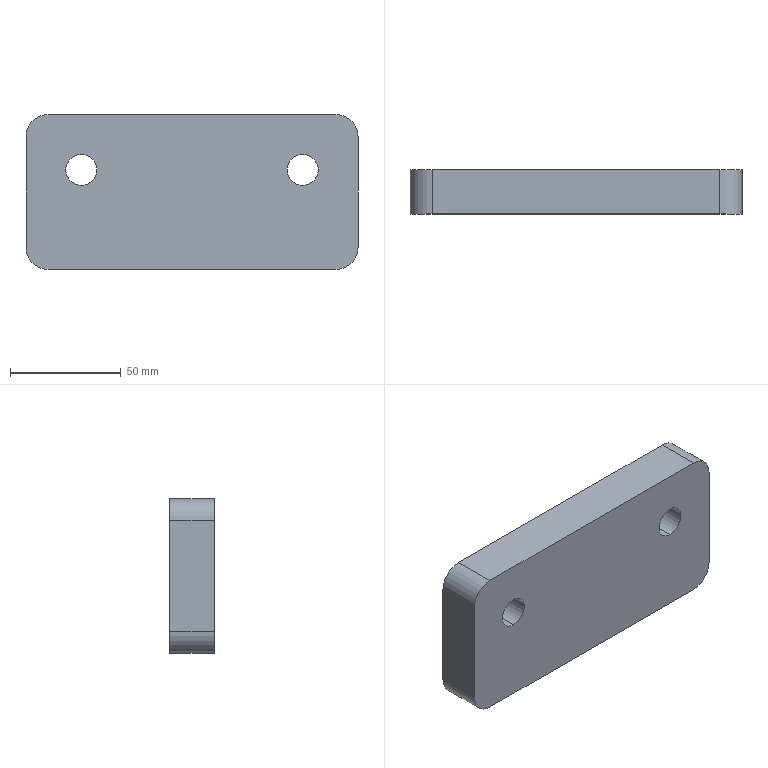Part | SolidWorks | features BaseBody 1 | 1 solid | 14 faces | box 150 x 20 x 70 mm | volume 202126 mm3 | cylinder 8 | plane 6 | commonest cylinder face diameters 14 x4 20 x4
STEP:
#1=CARTESIAN_POINT('',(-50.,-12.5,17.));
#2=VERTEX_POINT('',#1);
#3=CARTESIAN_POINT('',(-50.,-12.5,3.));
#4=VERTEX_POINT('',#3);
#5=CARTESIAN_POINT('',(-50.,-12.5,10.));
#6=DIRECTION('',(0.,-1.,0.));
#7=DIRECTION('',(0.,0.,-1.));
#8=AXIS2_PLACEMENT_3D('',#5,#6,#7);
#9=CIRCLE('',#8,7.);
#10=EDGE_CURVE('',#2,#4,#9,.T.);
#11=ORIENTED_EDGE('',*,*,#10,.T.);
#12=CARTESIAN_POINT('',(-50.,7.5,3.));
#13=VERTEX_POINT('',#12);
#14=CARTESIAN_POINT('',(-50.,7.5,3.));
#15=DIRECTION('',(0.,1.,0.));
#16=VECTOR('',#15,1000.);
#17=LINE('',#14,#16);
#18=EDGE_CURVE('',#4,#13,#17,.T.);
#19=ORIENTED_EDGE('',*,*,#18,.T.);
#20=CARTESIAN_POINT('',(-50.,7.5,17.));
#21=VERTEX_POINT('',#20);
#22=CARTESIAN_POINT('',(-50.,7.5,10.));
#23=DIRECTION('',(0.,1.,0.));
#24=DIRECTION('',(0.,0.,1.));
#25=AXIS2_PLACEMENT_3D('',#22,#23,#24);
#26=CIRCLE('',#25,7.);
#27=EDGE_CURVE('',#13,#21,#26,.T.);
#28=ORIENTED_EDGE('',*,*,#27,.T.);
#29=CARTESIAN_POINT('',(-50.,7.5,17.));
#30=DIRECTION('',(0.,1.,0.));
#31=VECTOR('',#30,1000.);
#32=LINE('',#29,#31);
#33=EDGE_CURVE('',#2,#21,#32,.T.);
#34=ORIENTED_EDGE('',*,*,#33,.F.);
#35=EDGE_LOOP('',(#11,#19,#28,#34));
#36=FACE_OUTER_BOUND('',#35,.T.);
#37=CARTESIAN_POINT('',(-50.,7.5,10.));
#38=DIRECTION('',(0.,1.,0.));
#39=DIRECTION('',(0.,0.,1.));
#40=AXIS2_PLACEMENT_3D('',#37,#38,#39);
#41=CYLINDRICAL_SURFACE('',#40,7.);
#42=ADVANCED_FACE('',(#36),#41,.F.);
#43=CARTESIAN_POINT('',(50.,-12.5,17.));
#44=VERTEX_POINT('',#43);
#45=CARTESIAN_POINT('',(50.,-12.5,3.));
#46=VERTEX_POINT('',#45);
#47=CARTESIAN_POINT('',(50.,-12.5,10.));
#48=DIRECTION('',(0.,-1.,0.));
#49=DIRECTION('',(0.,0.,-1.));
#50=AXIS2_PLACEMENT_3D('',#47,#48,#49);
#51=CIRCLE('',#50,7.);
#52=EDGE_CURVE('',#44,#46,#51,.T.);
#53=ORIENTED_EDGE('',*,*,#52,.T.);
#54=CARTESIAN_POINT('',(50.,7.5,3.));
#55=VERTEX_POINT('',#54);
#56=CARTESIAN_POINT('',(50.,7.5,3.));
#57=DIRECTION('',(0.,1.,0.));
#58=VECTOR('',#57,1000.);
#59=LINE('',#56,#58);
#60=EDGE_CURVE('',#46,#55,#59,.T.);
#61=ORIENTED_EDGE('',*,*,#60,.T.);
#62=CARTESIAN_POINT('',(50.,7.5,17.));
#63=VERTEX_POINT('',#62);
#64=CARTESIAN_POINT('',(50.,7.5,10.));
#65=DIRECTION('',(0.,1.,0.));
#66=DIRECTION('',(0.,0.,1.));
#67=AXIS2_PLACEMENT_3D('',#64,#65,#66);
#68=CIRCLE('',#67,7.);
#69=EDGE_CURVE('',#55,#63,#68,.T.);
#70=ORIENTED_EDGE('',*,*,#69,.T.);
#71=CARTESIAN_POINT('',(50.,7.5,17.));
#72=DIRECTION('',(0.,1.,0.));
#73=VECTOR('',#72,1000.);
#74=LINE('',#71,#73);
#75=EDGE_CURVE('',#44,#63,#74,.T.);
#76=ORIENTED_EDGE('',*,*,#75,.F.);
#77=EDGE_LOOP('',(#53,#61,#70,#76));
#78=FACE_OUTER_BOUND('',#77,.T.);
#79=CARTESIAN_POINT('',(50.,7.5,10.));
#80=DIRECTION('',(0.,1.,0.));
#81=DIRECTION('',(0.,0.,1.));
#82=AXIS2_PLACEMENT_3D('',#79,#80,#81);
#83=CYLINDRICAL_SURFACE('',#82,7.);
#84=ADVANCED_FACE('',(#78),#83,.F.);
#85=CARTESIAN_POINT('',(75.,7.5,-25.));
#86=VERTEX_POINT('',#85);
#87=CARTESIAN_POINT('',(65.,7.5,-35.));
#88=VERTEX_POINT('',#87);
#89=CARTESIAN_POINT('',(65.,7.5,-25.));
#90=DIRECTION('',(0.,1.,0.));
#91=DIRECTION('',(0.,0.,1.));
#92=AXIS2_PLACEMENT_3D('',#89,#90,#91);
#93=CIRCLE('',#92,10.);
#94=EDGE_CURVE('',#86,#88,#93,.T.);
#95=ORIENTED_EDGE('',*,*,#94,.F.);
#96=CARTESIAN_POINT('',(75.,-12.5,-25.));
#97=VERTEX_POINT('',#96);
#98=CARTESIAN_POINT('',(75.,12.5,-25.));
#99=DIRECTION('',(0.,-1.,0.));
#100=VECTOR('',#99,1000.);
#101=LINE('',#98,#100);
#102=EDGE_CURVE('',#86,#97,#101,.T.);
#103=ORIENTED_EDGE('',*,*,#102,.T.);
#104=CARTESIAN_POINT('',(65.,-12.5,-35.));
#105=VERTEX_POINT('',#104);
#106=CARTESIAN_POINT('',(65.,-12.5,-25.));
#107=DIRECTION('',(0.,1.,0.));
#108=DIRECTION('',(0.,0.,-1.));
#109=AXIS2_PLACEMENT_3D('',#106,#107,#108);
#110=CIRCLE('',#109,10.);
#111=EDGE_CURVE('',#97,#105,#110,.T.);
#112=ORIENTED_EDGE('',*,*,#111,.T.);
#113=CARTESIAN_POINT('',(65.,12.5,-35.));
#114=DIRECTION('',(0.,-1.,0.));
#115=VECTOR('',#114,1000.);
#116=LINE('',#113,#115);
#117=EDGE_CURVE('',#88,#105,#116,.T.);
#118=ORIENTED_EDGE('',*,*,#117,.F.);
#119=EDGE_LOOP('',(#95,#103,#112,#118));
#120=FACE_OUTER_BOUND('',#119,.T.);
#121=CARTESIAN_POINT('',(65.,12.5,-25.));
#122=DIRECTION('',(0.,-1.,0.));
#123=DIRECTION('',(0.,0.,-1.));
#124=AXIS2_PLACEMENT_3D('',#121,#122,#123);
#125=CYLINDRICAL_SURFACE('',#124,10.);
#126=ADVANCED_FACE('',(#120),#125,.T.);
#127=CARTESIAN_POINT('',(-65.,7.5,-35.));
#128=VERTEX_POINT('',#127);
#129=CARTESIAN_POINT('',(65.,7.5,-35.));
#130=DIRECTION('',(-1.,0.,0.));
#131=VECTOR('',#130,1000.);
#132=LINE('',#129,#131);
#133=EDGE_CURVE('',#88,#128,#132,.T.);
#134=ORIENTED_EDGE('',*,*,#133,.F.);
#135=ORIENTED_EDGE('',*,*,#117,.T.);
#136=CARTESIAN_POINT('',(-65.,-12.5,-35.));
#137=VERTEX_POINT('',#136);
#138=CARTESIAN_POINT('',(-65.,-12.5,-35.));
#139=DIRECTION('',(-1.,0.,0.));
#140=VECTOR('',#139,1000.);
#141=LINE('',#138,#140);
#142=EDGE_CURVE('',#105,#137,#141,.T.);
#143=ORIENTED_EDGE('',*,*,#142,.T.);
#144=CARTESIAN_POINT('',(-65.,12.5,-35.));
#145=DIRECTION('',(0.,-1.,0.));
#146=VECTOR('',#145,1000.);
#147=LINE('',#144,#146);
#148=EDGE_CURVE('',#128,#137,#147,.T.);
#149=ORIENTED_EDGE('',*,*,#148,.F.);
#150=EDGE_LOOP('',(#134,#135,#143,#149));
#151=FACE_OUTER_BOUND('',#150,.T.);
#152=CARTESIAN_POINT('',(-65.,12.5,-35.));
#153=DIRECTION('',(0.,0.,1.));
#154=DIRECTION('',(1.,0.,0.));
#155=AXIS2_PLACEMENT_3D('',#152,#153,#154);
#156=PLANE('',#155);
#157=ADVANCED_FACE('',(#151),#156,.F.);
#158=CARTESIAN_POINT('',(-75.,7.5,-25.));
#159=VERTEX_POINT('',#158);
#160=CARTESIAN_POINT('',(-65.,7.5,-25.));
#161=DIRECTION('',(0.,1.,0.));
#162=DIRECTION('',(0.,0.,1.));
#163=AXIS2_PLACEMENT_3D('',#160,#161,#162);
#164=CIRCLE('',#163,10.);
#165=EDGE_CURVE('',#128,#159,#164,.T.);
#166=ORIENTED_EDGE('',*,*,#165,.F.);
#167=ORIENTED_EDGE('',*,*,#148,.T.);
#168=CARTESIAN_POINT('',(-75.,-12.5,-25.));
#169=VERTEX_POINT('',#168);
#170=CARTESIAN_POINT('',(-65.,-12.5,-25.));
#171=DIRECTION('',(0.,1.,0.));
#172=DIRECTION('',(0.,0.,1.));
#173=AXIS2_PLACEMENT_3D('',#170,#171,#172);
#174=CIRCLE('',#173,10.);
#175=EDGE_CURVE('',#137,#169,#174,.T.);
#176=ORIENTED_EDGE('',*,*,#175,.T.);
#177=CARTESIAN_POINT('',(-75.,12.5,-25.));
#178=DIRECTION('',(0.,-1.,0.));
#179=VECTOR('',#178,1000.);
#180=LINE('',#177,#179);
#181=EDGE_CURVE('',#159,#169,#180,.T.);
#182=ORIENTED_EDGE('',*,*,#181,.F.);
#183=EDGE_LOOP('',(#166,#167,#176,#182));
#184=FACE_OUTER_BOUND('',#183,.T.);
#185=CARTESIAN_POINT('',(-65.,12.5,-25.));
#186=DIRECTION('',(0.,-1.,0.));
#187=DIRECTION('',(0.,0.,-1.));
#188=AXIS2_PLACEMENT_3D('',#185,#186,#187);
#189=CYLINDRICAL_SURFACE('',#188,10.);
#190=ADVANCED_FACE('',(#184),#189,.T.);
#191=CARTESIAN_POINT('',(-75.,7.5,25.));
#192=VERTEX_POINT('',#191);
#193=CARTESIAN_POINT('',(-75.,7.5,-25.));
#194=DIRECTION('',(0.,0.,1.));
#195=VECTOR('',#194,1000.);
#196=LINE('',#193,#195);
#197=EDGE_CURVE('',#159,#192,#196,.T.);
#198=ORIENTED_EDGE('',*,*,#197,.F.);
#199=ORIENTED_EDGE('',*,*,#181,.T.);
#200=CARTESIAN_POINT('',(-75.,-12.5,25.));
#201=VERTEX_POINT('',#200);
#202=CARTESIAN_POINT('',(-75.,-12.5,-25.));
#203=DIRECTION('',(0.,0.,1.));
#204=VECTOR('',#203,1000.);
#205=LINE('',#202,#204);
#206=EDGE_CURVE('',#169,#201,#205,.T.);
#207=ORIENTED_EDGE('',*,*,#206,.T.);
#208=CARTESIAN_POINT('',(-75.,12.5,25.));
#209=DIRECTION('',(0.,-1.,0.));
#210=VECTOR('',#209,1000.);
#211=LINE('',#208,#210);
#212=EDGE_CURVE('',#192,#201,#211,.T.);
#213=ORIENTED_EDGE('',*,*,#212,.F.);
#214=EDGE_LOOP('',(#198,#199,#207,#213));
#215=FACE_OUTER_BOUND('',#214,.T.);
#216=CARTESIAN_POINT('',(-75.,12.5,-25.));
#217=DIRECTION('',(1.,0.,0.));
#218=DIRECTION('',(0.,0.,-1.));
#219=AXIS2_PLACEMENT_3D('',#216,#217,#218);
#220=PLANE('',#219);
#221=ADVANCED_FACE('',(#215),#220,.F.);
#222=CARTESIAN_POINT('',(-65.,7.5,35.));
#223=VERTEX_POINT('',#222);
#224=CARTESIAN_POINT('',(-65.,7.5,25.));
#225=DIRECTION('',(0.,1.,0.));
#226=DIRECTION('',(0.,0.,1.));
#227=AXIS2_PLACEMENT_3D('',#224,#225,#226);
#228=CIRCLE('',#227,10.);
#229=EDGE_CURVE('',#192,#223,#228,.T.);
#230=ORIENTED_EDGE('',*,*,#229,.F.);
#231=ORIENTED_EDGE('',*,*,#212,.T.);
#232=CARTESIAN_POINT('',(-65.,-12.5,35.));
#233=VERTEX_POINT('',#232);
#234=CARTESIAN_POINT('',(-65.,-12.5,25.));
#235=DIRECTION('',(0.,1.,0.));
#236=DIRECTION('',(0.,0.,1.));
#237=AXIS2_PLACEMENT_3D('',#234,#235,#236);
#238=CIRCLE('',#237,10.);
#239=EDGE_CURVE('',#201,#233,#238,.T.);
#240=ORIENTED_EDGE('',*,*,#239,.T.);
#241=CARTESIAN_POINT('',(-65.,12.5,35.));
#242=DIRECTION('',(0.,-1.,0.));
#243=VECTOR('',#242,1000.);
#244=LINE('',#241,#243);
#245=EDGE_CURVE('',#223,#233,#244,.T.);
#246=ORIENTED_EDGE('',*,*,#245,.F.);
#247=EDGE_LOOP('',(#230,#231,#240,#246));
#248=FACE_OUTER_BOUND('',#247,.T.);
#249=CARTESIAN_POINT('',(-65.,12.5,25.));
#250=DIRECTION('',(0.,-1.,0.));
#251=DIRECTION('',(0.,0.,-1.));
#252=AXIS2_PLACEMENT_3D('',#249,#250,#251);
#253=CYLINDRICAL_SURFACE('',#252,10.);
#254=ADVANCED_FACE('',(#248),#253,.T.);
#255=CARTESIAN_POINT('',(65.,7.5,35.));
#256=VERTEX_POINT('',#255);
#257=CARTESIAN_POINT('',(-65.,7.5,35.));
#258=DIRECTION('',(1.,0.,0.));
#259=VECTOR('',#258,1000.);
#260=LINE('',#257,#259);
#261=EDGE_CURVE('',#223,#256,#260,.T.);
#262=ORIENTED_EDGE('',*,*,#261,.F.);
#263=ORIENTED_EDGE('',*,*,#245,.T.);
#264=CARTESIAN_POINT('',(65.,-12.5,35.));
#265=VERTEX_POINT('',#264);
#266=CARTESIAN_POINT('',(-65.,-12.5,35.));
#267=DIRECTION('',(1.,0.,0.));
#268=VECTOR('',#267,1000.);
#269=LINE('',#266,#268);
#270=EDGE_CURVE('',#233,#265,#269,.T.);
#271=ORIENTED_EDGE('',*,*,#270,.T.);
#272=CARTESIAN_POINT('',(65.,12.5,35.));
#273=DIRECTION('',(0.,-1.,0.));
#274=VECTOR('',#273,1000.);
#275=LINE('',#272,#274);
#276=EDGE_CURVE('',#256,#265,#275,.T.);
#277=ORIENTED_EDGE('',*,*,#276,.F.);
#278=EDGE_LOOP('',(#262,#263,#271,#277));
#279=FACE_OUTER_BOUND('',#278,.T.);
#280=CARTESIAN_POINT('',(-65.,12.5,35.));
#281=DIRECTION('',(0.,0.,-1.));
#282=DIRECTION('',(-1.,0.,0.));
#283=AXIS2_PLACEMENT_3D('',#280,#281,#282);
#284=PLANE('',#283);
#285=ADVANCED_FACE('',(#279),#284,.F.);
#286=CARTESIAN_POINT('',(75.,7.5,25.));
#287=VERTEX_POINT('',#286);
#288=CARTESIAN_POINT('',(65.,7.5,25.));
#289=DIRECTION('',(0.,1.,0.));
#290=DIRECTION('',(0.,0.,1.));
#291=AXIS2_PLACEMENT_3D('',#288,#289,#290);
#292=CIRCLE('',#291,10.);
#293=EDGE_CURVE('',#256,#287,#292,.T.);
#294=ORIENTED_EDGE('',*,*,#293,.F.);
#295=ORIENTED_EDGE('',*,*,#276,.T.);
#296=CARTESIAN_POINT('',(75.,-12.5,25.));
#297=VERTEX_POINT('',#296);
#298=CARTESIAN_POINT('',(65.,-12.5,25.));
#299=DIRECTION('',(0.,1.,0.));
#300=DIRECTION('',(0.,0.,1.));
#301=AXIS2_PLACEMENT_3D('',#298,#299,#300);
#302=CIRCLE('',#301,10.);
#303=EDGE_CURVE('',#265,#297,#302,.T.);
#304=ORIENTED_EDGE('',*,*,#303,.T.);
#305=CARTESIAN_POINT('',(75.,12.5,25.));
#306=DIRECTION('',(0.,-1.,0.));
#307=VECTOR('',#306,1000.);
#308=LINE('',#305,#307);
#309=EDGE_CURVE('',#287,#297,#308,.T.);
#310=ORIENTED_EDGE('',*,*,#309,.F.);
#311=EDGE_LOOP('',(#294,#295,#304,#310));
#312=FACE_OUTER_BOUND('',#311,.T.);
#313=CARTESIAN_POINT('',(65.,12.5,25.));
#314=DIRECTION('',(0.,-1.,0.));
#315=DIRECTION('',(0.,0.,-1.));
#316=AXIS2_PLACEMENT_3D('',#313,#314,#315);
#317=CYLINDRICAL_SURFACE('',#316,10.);
#318=ADVANCED_FACE('',(#312),#317,.T.);
#319=CARTESIAN_POINT('',(75.,7.5,25.));
#320=DIRECTION('',(0.,0.,-1.));
#321=VECTOR('',#320,1000.);
#322=LINE('',#319,#321);
#323=EDGE_CURVE('',#287,#86,#322,.T.);
#324=ORIENTED_EDGE('',*,*,#323,.F.);
#325=ORIENTED_EDGE('',*,*,#309,.T.);
#326=CARTESIAN_POINT('',(75.,-12.5,-25.));
#327=DIRECTION('',(0.,0.,-1.));
#328=VECTOR('',#327,1000.);
#329=LINE('',#326,#328);
#330=EDGE_CURVE('',#297,#97,#329,.T.);
#331=ORIENTED_EDGE('',*,*,#330,.T.);
#332=ORIENTED_EDGE('',*,*,#102,.F.);
#333=EDGE_LOOP('',(#324,#325,#331,#332));
#334=FACE_OUTER_BOUND('',#333,.T.);
#335=CARTESIAN_POINT('',(75.,12.5,-25.));
#336=DIRECTION('',(-1.,0.,0.));
#337=DIRECTION('',(0.,0.,1.));
#338=AXIS2_PLACEMENT_3D('',#335,#336,#337);
#339=PLANE('',#338);
#340=ADVANCED_FACE('',(#334),#339,.F.);
#341=ORIENTED_EDGE('',*,*,#10,.F.);
#342=CARTESIAN_POINT('',(-50.,-12.5,10.));
#343=DIRECTION('',(0.,-1.,0.));
#344=DIRECTION('',(0.,0.,-1.));
#345=AXIS2_PLACEMENT_3D('',#342,#343,#344);
#346=CIRCLE('',#345,7.);
#347=EDGE_CURVE('',#4,#2,#346,.T.);
#348=ORIENTED_EDGE('',*,*,#347,.F.);
#349=EDGE_LOOP('',(#341,#348));
#350=FACE_BOUND('',#349,.T.);
#351=ORIENTED_EDGE('',*,*,#52,.F.);
#352=CARTESIAN_POINT('',(50.,-12.5,10.));
#353=DIRECTION('',(0.,-1.,0.));
#354=DIRECTION('',(0.,0.,-1.));
#355=AXIS2_PLACEMENT_3D('',#352,#353,#354);
#356=CIRCLE('',#355,7.);
#357=EDGE_CURVE('',#46,#44,#356,.T.);
#358=ORIENTED_EDGE('',*,*,#357,.F.);
#359=EDGE_LOOP('',(#351,#358));
#360=FACE_BOUND('',#359,.T.);
#361=ORIENTED_EDGE('',*,*,#111,.F.);
#362=ORIENTED_EDGE('',*,*,#330,.F.);
#363=ORIENTED_EDGE('',*,*,#303,.F.);
#364=ORIENTED_EDGE('',*,*,#270,.F.);
#365=ORIENTED_EDGE('',*,*,#239,.F.);
#366=ORIENTED_EDGE('',*,*,#206,.F.);
#367=ORIENTED_EDGE('',*,*,#175,.F.);
#368=ORIENTED_EDGE('',*,*,#142,.F.);
#369=EDGE_LOOP('',(#361,#362,#363,#364,#365,#366,#367,#368));
#370=FACE_OUTER_BOUND('',#369,.T.);
#371=CARTESIAN_POINT('',(65.,-12.5,-25.));
#372=DIRECTION('',(0.,-1.,0.));
#373=DIRECTION('',(0.,0.,-1.));
#374=AXIS2_PLACEMENT_3D('',#371,#372,#373);
#375=PLANE('',#374);
#376=ADVANCED_FACE('',(#350,#360,#370),#375,.T.);
#377=CARTESIAN_POINT('',(-50.,7.5,10.));
#378=DIRECTION('',(0.,1.,0.));
#379=DIRECTION('',(0.,0.,1.));
#380=AXIS2_PLACEMENT_3D('',#377,#378,#379);
#381=CIRCLE('',#380,7.);
#382=EDGE_CURVE('',#21,#13,#381,.T.);
#383=ORIENTED_EDGE('',*,*,#382,.F.);
#384=ORIENTED_EDGE('',*,*,#27,.F.);
#385=EDGE_LOOP('',(#383,#384));
#386=FACE_BOUND('',#385,.T.);
#387=CARTESIAN_POINT('',(50.,7.5,10.));
#388=DIRECTION('',(0.,1.,0.));
#389=DIRECTION('',(0.,0.,1.));
#390=AXIS2_PLACEMENT_3D('',#387,#388,#389);
#391=CIRCLE('',#390,7.);
#392=EDGE_CURVE('',#63,#55,#391,.T.);
#393=ORIENTED_EDGE('',*,*,#392,.F.);
#394=ORIENTED_EDGE('',*,*,#69,.F.);
#395=EDGE_LOOP('',(#393,#394));
#396=FACE_BOUND('',#395,.T.);
#397=ORIENTED_EDGE('',*,*,#94,.T.);
#398=ORIENTED_EDGE('',*,*,#133,.T.);
#399=ORIENTED_EDGE('',*,*,#165,.T.);
#400=ORIENTED_EDGE('',*,*,#197,.T.);
#401=ORIENTED_EDGE('',*,*,#229,.T.);
#402=ORIENTED_EDGE('',*,*,#261,.T.);
#403=ORIENTED_EDGE('',*,*,#293,.T.);
#404=ORIENTED_EDGE('',*,*,#323,.T.);
#405=EDGE_LOOP('',(#397,#398,#399,#400,#401,#402,#403,#404));
#406=FACE_OUTER_BOUND('',#405,.T.);
#407=CARTESIAN_POINT('',(65.,7.5,-25.));
#408=DIRECTION('',(0.,1.,0.));
#409=DIRECTION('',(0.,0.,1.));
#410=AXIS2_PLACEMENT_3D('',#407,#408,#409);
#411=PLANE('',#410);
#412=ADVANCED_FACE('',(#386,#396,#406),#411,.T.);
#413=ORIENTED_EDGE('',*,*,#60,.F.);
#414=ORIENTED_EDGE('',*,*,#357,.T.);
#415=ORIENTED_EDGE('',*,*,#75,.T.);
#416=ORIENTED_EDGE('',*,*,#392,.T.);
#417=EDGE_LOOP('',(#413,#414,#415,#416));
#418=FACE_OUTER_BOUND('',#417,.T.);
#419=CARTESIAN_POINT('',(50.,7.5,10.));
#420=DIRECTION('',(0.,1.,0.));
#421=DIRECTION('',(0.,0.,1.));
#422=AXIS2_PLACEMENT_3D('',#419,#420,#421);
#423=CYLINDRICAL_SURFACE('',#422,7.);
#424=ADVANCED_FACE('',(#418),#423,.F.);
#425=ORIENTED_EDGE('',*,*,#18,.F.);
#426=ORIENTED_EDGE('',*,*,#347,.T.);
#427=ORIENTED_EDGE('',*,*,#33,.T.);
#428=ORIENTED_EDGE('',*,*,#382,.T.);
#429=EDGE_LOOP('',(#425,#426,#427,#428));
#430=FACE_OUTER_BOUND('',#429,.T.);
#431=CARTESIAN_POINT('',(-50.,7.5,10.));
#432=DIRECTION('',(0.,1.,0.));
#433=DIRECTION('',(0.,0.,1.));
#434=AXIS2_PLACEMENT_3D('',#431,#432,#433);
#435=CYLINDRICAL_SURFACE('',#434,7.);
#436=ADVANCED_FACE('',(#430),#435,.F.);
#437=CLOSED_SHELL('',(#42,#84,#126,#157,#190,#221,#254,#285,#318,#340,#376,#412,#424,#436));
#438=MANIFOLD_SOLID_BREP('',#437);
#439=CARTESIAN_POINT('',(0.,0.,0.));
#440=DIRECTION('',(0.,0.,1.));
#441=DIRECTION('',(1.,0.,0.));
#442=AXIS2_PLACEMENT_3D('',#439,#440,#441);
#443=(LENGTH_UNIT()NAMED_UNIT(*)SI_UNIT(.MILLI.,.METRE.));
#444=UNCERTAINTY_MEASURE_WITH_UNIT(LENGTH_MEASURE(0.00001),#443,'','');
#445=(NAMED_UNIT(*)PLANE_ANGLE_UNIT()SI_UNIT($,.RADIAN.));
#446=(NAMED_UNIT(*)SI_UNIT($,.STERADIAN.)SOLID_ANGLE_UNIT());
#447=(GEOMETRIC_REPRESENTATION_CONTEXT(3)GLOBAL_UNCERTAINTY_ASSIGNED_CONTEXT((#444))GLOBAL_UNIT_ASSIGNED_CONTEXT((#443,#445,#446))REPRESENTATION_CONTEXT('',''));
#448=ADVANCED_BREP_SHAPE_REPRESENTATION('',(#438,#442),#447);